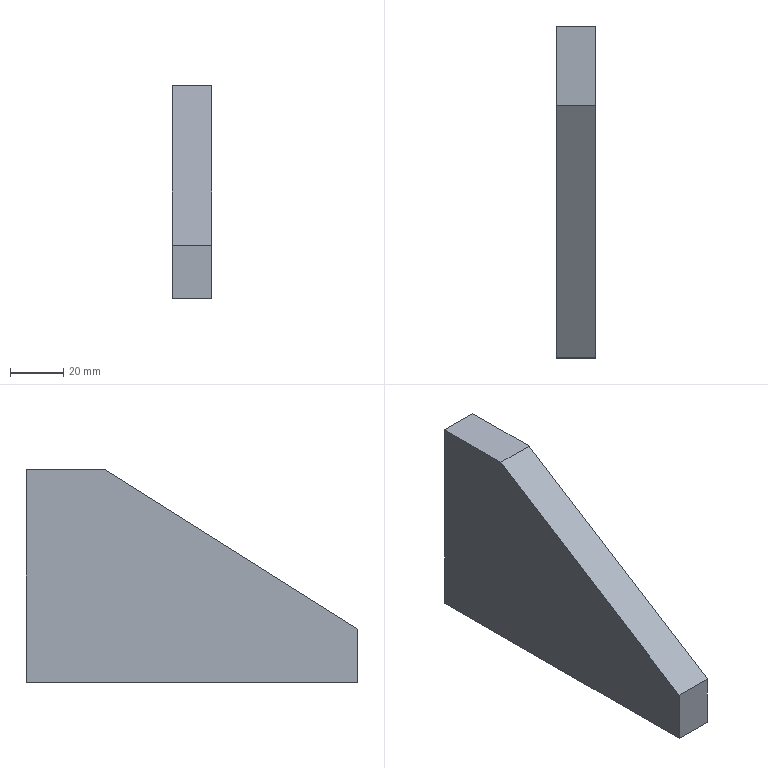Part | SolidWorks | features Extrusion 1 | 1 solid | 7 faces | box 15 x 125 x 80 mm | volume 107250 mm3 | plane 7
STEP:
#1=CARTESIAN_POINT('',(-7.5,0.,20.));
#2=VERTEX_POINT('',#1);
#3=CARTESIAN_POINT('',(-7.5,0.,0.));
#4=VERTEX_POINT('',#3);
#5=CARTESIAN_POINT('',(-7.5,0.,20.));
#6=DIRECTION('',(0.,0.,-1.));
#7=VECTOR('',#6,1000.);
#8=LINE('',#5,#7);
#9=EDGE_CURVE('',#2,#4,#8,.T.);
#10=ORIENTED_EDGE('',*,*,#9,.T.);
#11=CARTESIAN_POINT('',(7.5,0.,0.));
#12=VERTEX_POINT('',#11);
#13=CARTESIAN_POINT('',(7.5,0.,0.));
#14=DIRECTION('',(-1.,0.,0.));
#15=VECTOR('',#14,1000.);
#16=LINE('',#13,#15);
#17=EDGE_CURVE('',#12,#4,#16,.T.);
#18=ORIENTED_EDGE('',*,*,#17,.F.);
#19=CARTESIAN_POINT('',(7.5,0.,20.));
#20=VERTEX_POINT('',#19);
#21=CARTESIAN_POINT('',(7.5,0.,20.));
#22=DIRECTION('',(0.,0.,-1.));
#23=VECTOR('',#22,1000.);
#24=LINE('',#21,#23);
#25=EDGE_CURVE('',#20,#12,#24,.T.);
#26=ORIENTED_EDGE('',*,*,#25,.F.);
#27=CARTESIAN_POINT('',(7.5,0.,20.));
#28=DIRECTION('',(-1.,0.,0.));
#29=VECTOR('',#28,1000.);
#30=LINE('',#27,#29);
#31=EDGE_CURVE('',#20,#2,#30,.T.);
#32=ORIENTED_EDGE('',*,*,#31,.T.);
#33=EDGE_LOOP('',(#10,#18,#26,#32));
#34=FACE_OUTER_BOUND('',#33,.T.);
#35=CARTESIAN_POINT('',(7.5,0.,20.));
#36=DIRECTION('',(0.,1.,0.));
#37=DIRECTION('',(0.,0.,1.));
#38=AXIS2_PLACEMENT_3D('',#35,#36,#37);
#39=PLANE('',#38);
#40=ADVANCED_FACE('',(#34),#39,.F.);
#41=CARTESIAN_POINT('',(-7.5,125.,0.));
#42=VERTEX_POINT('',#41);
#43=CARTESIAN_POINT('',(-7.5,0.,0.));
#44=DIRECTION('',(0.,1.,0.));
#45=VECTOR('',#44,1000.);
#46=LINE('',#43,#45);
#47=EDGE_CURVE('',#4,#42,#46,.T.);
#48=ORIENTED_EDGE('',*,*,#47,.T.);
#49=CARTESIAN_POINT('',(7.5,125.,0.));
#50=VERTEX_POINT('',#49);
#51=CARTESIAN_POINT('',(7.5,125.,0.));
#52=DIRECTION('',(-1.,0.,0.));
#53=VECTOR('',#52,1000.);
#54=LINE('',#51,#53);
#55=EDGE_CURVE('',#50,#42,#54,.T.);
#56=ORIENTED_EDGE('',*,*,#55,.F.);
#57=CARTESIAN_POINT('',(7.5,0.,0.));
#58=DIRECTION('',(0.,1.,0.));
#59=VECTOR('',#58,1000.);
#60=LINE('',#57,#59);
#61=EDGE_CURVE('',#12,#50,#60,.T.);
#62=ORIENTED_EDGE('',*,*,#61,.F.);
#63=ORIENTED_EDGE('',*,*,#17,.T.);
#64=EDGE_LOOP('',(#48,#56,#62,#63));
#65=FACE_OUTER_BOUND('',#64,.T.);
#66=CARTESIAN_POINT('',(7.5,0.,0.));
#67=DIRECTION('',(0.,0.,1.));
#68=DIRECTION('',(1.,0.,0.));
#69=AXIS2_PLACEMENT_3D('',#66,#67,#68);
#70=PLANE('',#69);
#71=ADVANCED_FACE('',(#65),#70,.F.);
#72=CARTESIAN_POINT('',(-7.5,125.,80.));
#73=VERTEX_POINT('',#72);
#74=CARTESIAN_POINT('',(-7.5,125.,0.));
#75=DIRECTION('',(0.,0.,1.));
#76=VECTOR('',#75,1000.);
#77=LINE('',#74,#76);
#78=EDGE_CURVE('',#42,#73,#77,.T.);
#79=ORIENTED_EDGE('',*,*,#78,.T.);
#80=CARTESIAN_POINT('',(7.5,125.,80.));
#81=VERTEX_POINT('',#80);
#82=CARTESIAN_POINT('',(7.5,125.,80.));
#83=DIRECTION('',(-1.,0.,0.));
#84=VECTOR('',#83,1000.);
#85=LINE('',#82,#84);
#86=EDGE_CURVE('',#81,#73,#85,.T.);
#87=ORIENTED_EDGE('',*,*,#86,.F.);
#88=CARTESIAN_POINT('',(7.5,125.,0.));
#89=DIRECTION('',(0.,0.,1.));
#90=VECTOR('',#89,1000.);
#91=LINE('',#88,#90);
#92=EDGE_CURVE('',#50,#81,#91,.T.);
#93=ORIENTED_EDGE('',*,*,#92,.F.);
#94=ORIENTED_EDGE('',*,*,#55,.T.);
#95=EDGE_LOOP('',(#79,#87,#93,#94));
#96=FACE_OUTER_BOUND('',#95,.T.);
#97=CARTESIAN_POINT('',(7.5,125.,0.));
#98=DIRECTION('',(0.,-1.,0.));
#99=DIRECTION('',(0.,0.,-1.));
#100=AXIS2_PLACEMENT_3D('',#97,#98,#99);
#101=PLANE('',#100);
#102=ADVANCED_FACE('',(#96),#101,.F.);
#103=CARTESIAN_POINT('',(-7.5,95.,80.));
#104=VERTEX_POINT('',#103);
#105=CARTESIAN_POINT('',(-7.5,125.,80.));
#106=DIRECTION('',(0.,-1.,0.));
#107=VECTOR('',#106,1000.);
#108=LINE('',#105,#107);
#109=EDGE_CURVE('',#73,#104,#108,.T.);
#110=ORIENTED_EDGE('',*,*,#109,.T.);
#111=CARTESIAN_POINT('',(7.5,95.,80.));
#112=VERTEX_POINT('',#111);
#113=CARTESIAN_POINT('',(7.5,95.,80.));
#114=DIRECTION('',(-1.,0.,0.));
#115=VECTOR('',#114,1000.);
#116=LINE('',#113,#115);
#117=EDGE_CURVE('',#112,#104,#116,.T.);
#118=ORIENTED_EDGE('',*,*,#117,.F.);
#119=CARTESIAN_POINT('',(7.5,125.,80.));
#120=DIRECTION('',(0.,-1.,0.));
#121=VECTOR('',#120,1000.);
#122=LINE('',#119,#121);
#123=EDGE_CURVE('',#81,#112,#122,.T.);
#124=ORIENTED_EDGE('',*,*,#123,.F.);
#125=ORIENTED_EDGE('',*,*,#86,.T.);
#126=EDGE_LOOP('',(#110,#118,#124,#125));
#127=FACE_OUTER_BOUND('',#126,.T.);
#128=CARTESIAN_POINT('',(7.5,125.,80.));
#129=DIRECTION('',(0.,0.,-1.));
#130=DIRECTION('',(0.,1.,0.));
#131=AXIS2_PLACEMENT_3D('',#128,#129,#130);
#132=PLANE('',#131);
#133=ADVANCED_FACE('',(#127),#132,.F.);
#134=CARTESIAN_POINT('',(-7.5,95.,80.));
#135=DIRECTION('',(0.,-0.8455,-0.534));
#136=VECTOR('',#135,1000.);
#137=LINE('',#134,#136);
#138=EDGE_CURVE('',#104,#2,#137,.T.);
#139=ORIENTED_EDGE('',*,*,#138,.T.);
#140=ORIENTED_EDGE('',*,*,#31,.F.);
#141=CARTESIAN_POINT('',(7.5,95.,80.));
#142=DIRECTION('',(0.,-0.8455,-0.534));
#143=VECTOR('',#142,1000.);
#144=LINE('',#141,#143);
#145=EDGE_CURVE('',#112,#20,#144,.T.);
#146=ORIENTED_EDGE('',*,*,#145,.F.);
#147=ORIENTED_EDGE('',*,*,#117,.T.);
#148=EDGE_LOOP('',(#139,#140,#146,#147));
#149=FACE_OUTER_BOUND('',#148,.T.);
#150=CARTESIAN_POINT('',(7.5,95.,80.));
#151=DIRECTION('',(0.,0.534,-0.8455));
#152=DIRECTION('',(0.,0.8455,0.534));
#153=AXIS2_PLACEMENT_3D('',#150,#151,#152);
#154=PLANE('',#153);
#155=ADVANCED_FACE('',(#149),#154,.F.);
#156=ORIENTED_EDGE('',*,*,#25,.T.);
#157=ORIENTED_EDGE('',*,*,#61,.T.);
#158=ORIENTED_EDGE('',*,*,#92,.T.);
#159=ORIENTED_EDGE('',*,*,#123,.T.);
#160=ORIENTED_EDGE('',*,*,#145,.T.);
#161=EDGE_LOOP('',(#156,#157,#158,#159,#160));
#162=FACE_OUTER_BOUND('',#161,.T.);
#163=CARTESIAN_POINT('',(7.5,0.,0.));
#164=DIRECTION('',(1.,0.,0.));
#165=DIRECTION('',(0.,0.,-1.));
#166=AXIS2_PLACEMENT_3D('',#163,#164,#165);
#167=PLANE('',#166);
#168=ADVANCED_FACE('',(#162),#167,.T.);
#169=ORIENTED_EDGE('',*,*,#9,.F.);
#170=ORIENTED_EDGE('',*,*,#138,.F.);
#171=ORIENTED_EDGE('',*,*,#109,.F.);
#172=ORIENTED_EDGE('',*,*,#78,.F.);
#173=ORIENTED_EDGE('',*,*,#47,.F.);
#174=EDGE_LOOP('',(#169,#170,#171,#172,#173));
#175=FACE_OUTER_BOUND('',#174,.T.);
#176=CARTESIAN_POINT('',(-7.5,0.,0.));
#177=DIRECTION('',(1.,0.,0.));
#178=DIRECTION('',(0.,0.,-1.));
#179=AXIS2_PLACEMENT_3D('',#176,#177,#178);
#180=PLANE('',#179);
#181=ADVANCED_FACE('',(#175),#180,.F.);
#182=CLOSED_SHELL('',(#40,#71,#102,#133,#155,#168,#181));
#183=MANIFOLD_SOLID_BREP('',#182);
#184=CARTESIAN_POINT('',(0.,0.,0.));
#185=DIRECTION('',(0.,0.,1.));
#186=DIRECTION('',(1.,0.,0.));
#187=AXIS2_PLACEMENT_3D('',#184,#185,#186);
#188=(LENGTH_UNIT()NAMED_UNIT(*)SI_UNIT(.MILLI.,.METRE.));
#189=UNCERTAINTY_MEASURE_WITH_UNIT(LENGTH_MEASURE(0.00001),#188,'','');
#190=(NAMED_UNIT(*)PLANE_ANGLE_UNIT()SI_UNIT($,.RADIAN.));
#191=(NAMED_UNIT(*)SI_UNIT($,.STERADIAN.)SOLID_ANGLE_UNIT());
#192=(GEOMETRIC_REPRESENTATION_CONTEXT(3)GLOBAL_UNCERTAINTY_ASSIGNED_CONTEXT((#189))GLOBAL_UNIT_ASSIGNED_CONTEXT((#188,#190,#191))REPRESENTATION_CONTEXT('',''));
#193=ADVANCED_BREP_SHAPE_REPRESENTATION('',(#183,#187),#192);